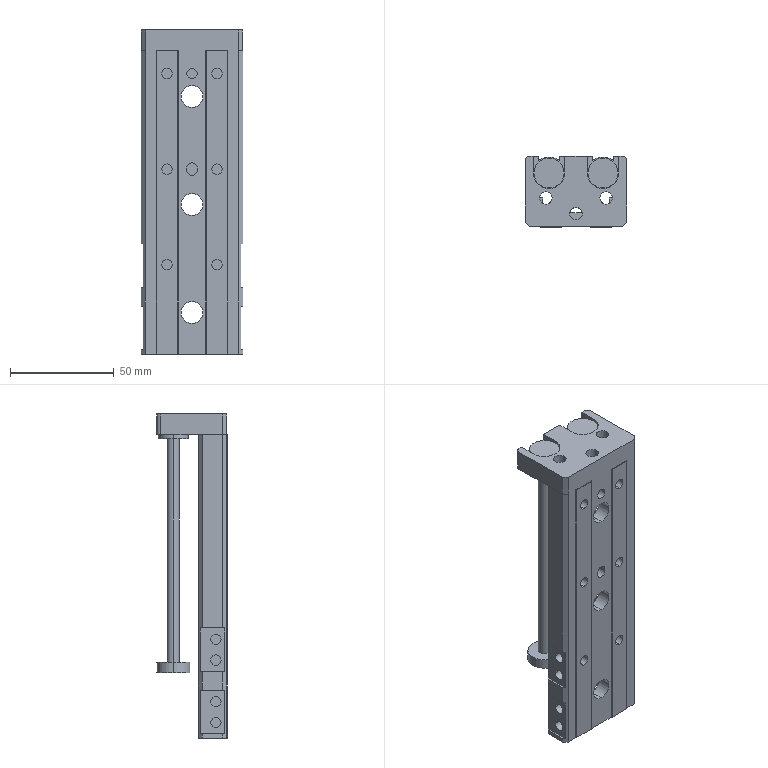Part | NX | 1 solid | 157 faces | box 49 x 34 x 156 mm | volume 83773 mm3 | plane 91 | cylinder 66 | commonest cylinder face diameters 5 x32 6 x10 14.5 x8 10.5 x6 15.9 x4 4 x2